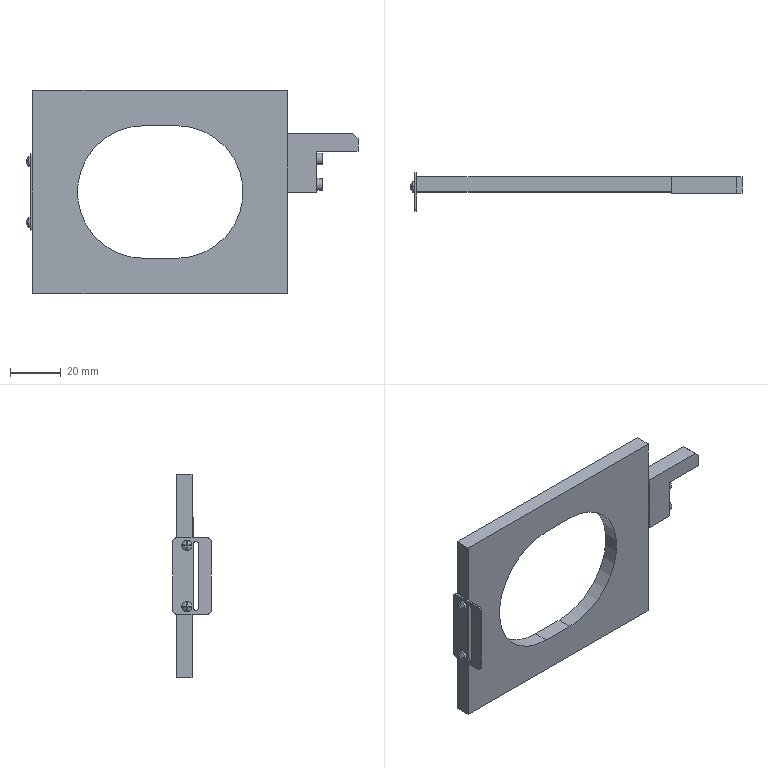Part | SolidWorks | features ICE 9, Revolution 2, Extrusion 1 | 1 solid | 86 faces | box 130.282 x 15 x 80 mm | volume 34016 mm3 | plane 61 | cylinder 17 | torus 8 | commonest cylinder face diameters 3 x4 4 x4 4.5 x4 2 x3 52 x2